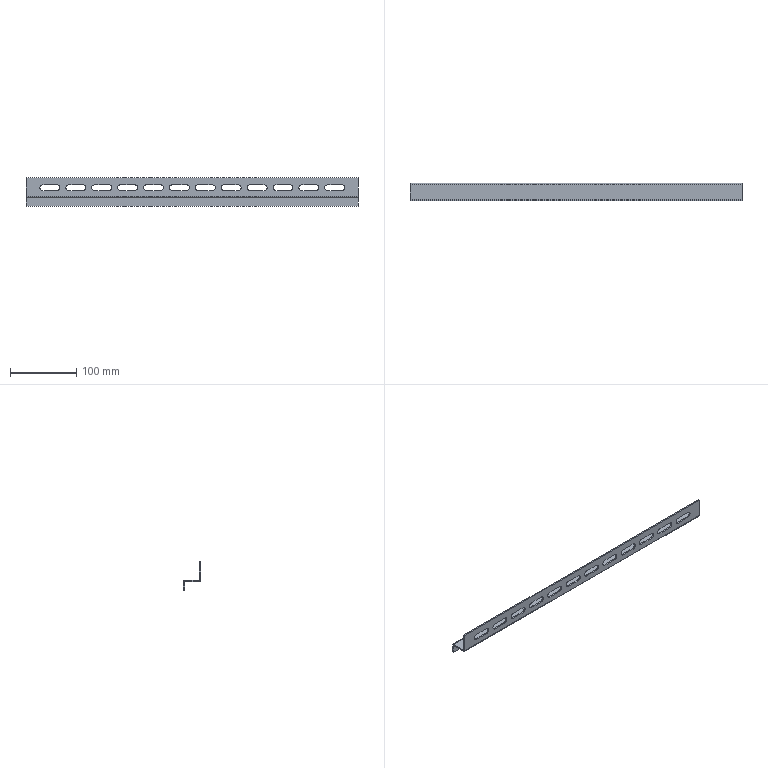Part | SolidWorks | features EdgeFlange 2, FlatPattern 1, ICE 1, LPattern 1, SMBaseFlange 1, SheetMetal 1 | 1 solid | 70 faces | box 500 x 26 x 43 mm | volume 59993 mm3 | plane 42 | cylinder 28 | commonest cylinder face diameters 9 x24 0.2 x2 4.2 x2